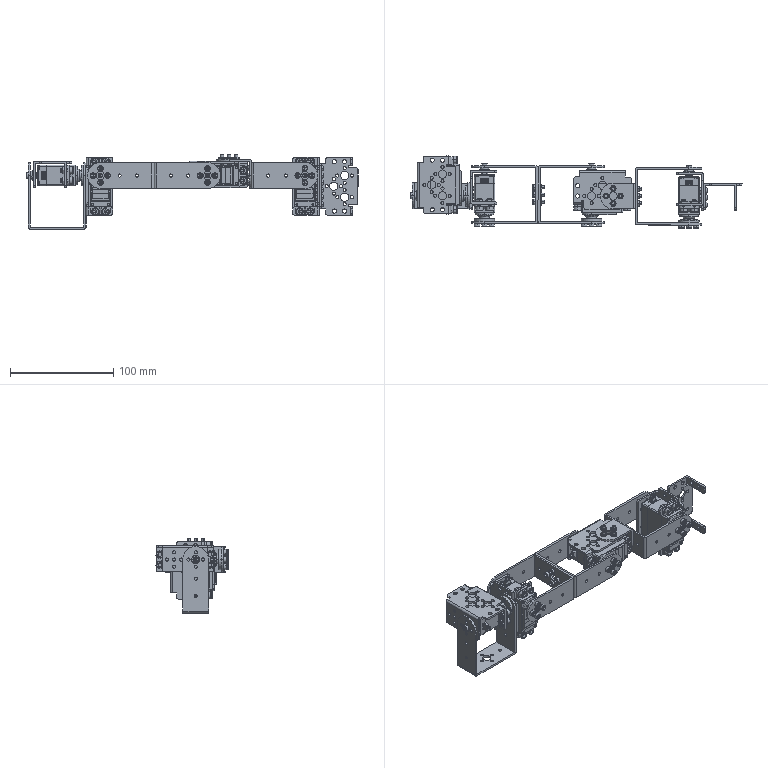Part | SolidWorks | features CompositeCurve 8 | 154 solids | 4842 faces | volume 161976 mm3 | plane 2158 | cylinder 1628 | cone 512 | torus 424 | spline 80 | sphere 40 | commonest cylinder face diameters 3 x476 4 x226 0.4 x208 2 x144 8 x66 1 x64